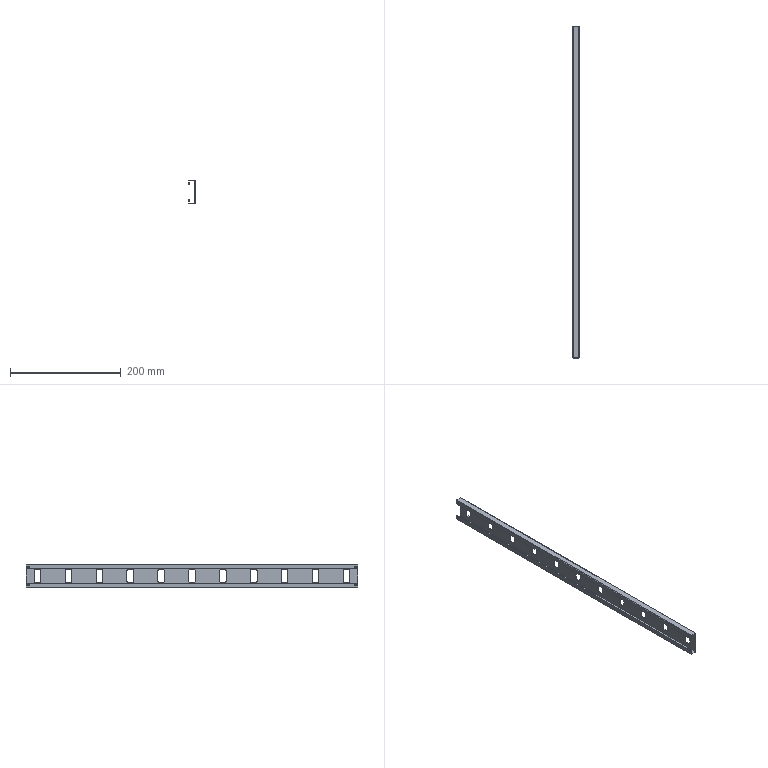Part | STEP file | HESS-408-70-15W-N-14-inner liner partition bracket | 1 solid | 122 faces | box 12 x 600 x 42 mm | volume 43540 mm3 | cylinder 64 | plane 58 | commonest cylinder face diameters 0.8 x44 3.2 x8 0.1 x4 2 x4 2.1 x4